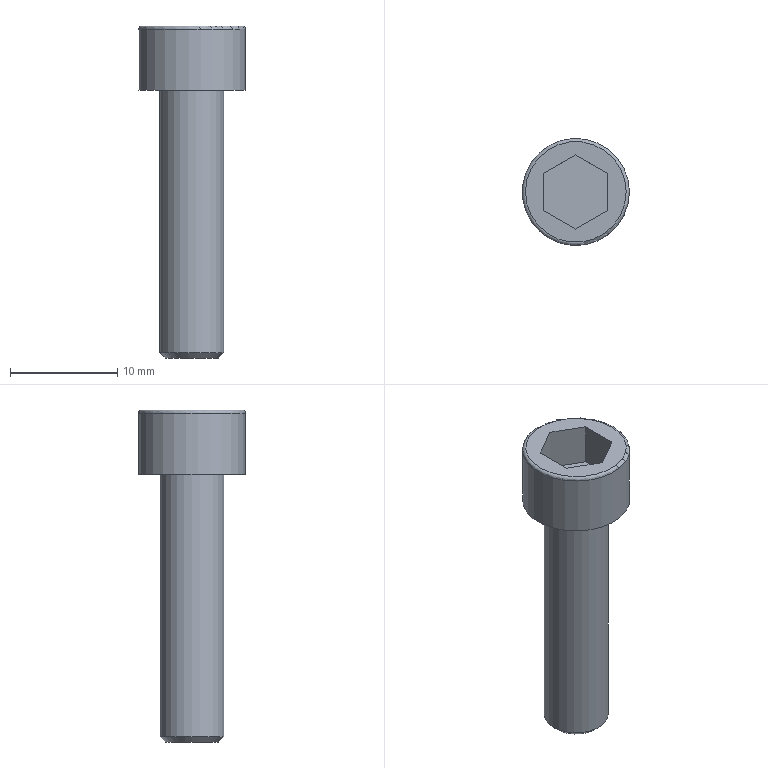Part | STEP file | 200 mesh_id622_x | 1 solid | 14 faces | box 10 x 10 x 31 mm | volume 1051 mm3 | plane 10 | cylinder 2 | torus 1 | cone 1 | commonest cylinder face diameters 6 x1 10 x1
STEP:
#1=CARTESIAN_POINT('',(-16735.684,-4117.769,77.5));
#2=VERTEX_POINT('',#1);
#3=CARTESIAN_POINT('',(-16732.684,-4117.769,77.5));
#4=DIRECTION('',(0.,0.,1.));
#5=DIRECTION('',(-1.,0.,0.));
#6=AXIS2_PLACEMENT_3D('',#3,#4,#5);
#7=CIRCLE('',#6,3.);
#8=EDGE_CURVE('',#2,#2,#7,.T.);
#9=ORIENTED_EDGE('',*,*,#8,.T.);
#10=EDGE_LOOP('',(#9));
#11=FACE_BOUND('',#10,.T.);
#12=CARTESIAN_POINT('',(-16735.684,-4117.769,102.));
#13=VERTEX_POINT('',#12);
#14=CARTESIAN_POINT('',(-16732.684,-4117.769,102.));
#15=DIRECTION('',(0.,0.,-1.));
#16=DIRECTION('',(-1.,0.,0.));
#17=AXIS2_PLACEMENT_3D('',#14,#15,#16);
#18=CIRCLE('',#17,3.);
#19=EDGE_CURVE('',#13,#13,#18,.T.);
#20=ORIENTED_EDGE('',*,*,#19,.T.);
#21=EDGE_LOOP('',(#20));
#22=FACE_BOUND('',#21,.T.);
#23=CARTESIAN_POINT('',(-16732.684,-4117.769,102.));
#24=DIRECTION('',(0.,0.,-1.));
#25=DIRECTION('',(1.,0.,0.));
#26=AXIS2_PLACEMENT_3D('',#23,#24,#25);
#27=CYLINDRICAL_SURFACE('',#26,3.);
#28=ADVANCED_FACE('',(#11,#22),#27,.T.);
#29=CARTESIAN_POINT('',(-16727.984,-4117.769,108.));
#30=VERTEX_POINT('',#29);
#31=CARTESIAN_POINT('',(-16732.684,-4117.769,108.));
#32=DIRECTION('',(0.,0.,-1.));
#33=DIRECTION('',(1.,0.,0.));
#34=AXIS2_PLACEMENT_3D('',#31,#32,#33);
#35=CIRCLE('',#34,4.7);
#36=EDGE_CURVE('',#30,#30,#35,.T.);
#37=ORIENTED_EDGE('',*,*,#36,.F.);
#38=EDGE_LOOP('',(#37));
#39=FACE_BOUND('',#38,.T.);
#40=CARTESIAN_POINT('',(-16735.684,-4119.501,108.));
#41=VERTEX_POINT('',#40);
#42=CARTESIAN_POINT('',(-16735.684,-4116.037,108.));
#43=VERTEX_POINT('',#42);
#44=CARTESIAN_POINT('',(-16735.684,-4119.501,108.));
#45=DIRECTION('',(0.,1.,0.));
#46=VECTOR('',#45,1.);
#47=LINE('',#44,#46);
#48=EDGE_CURVE('',#41,#43,#47,.T.);
#49=ORIENTED_EDGE('',*,*,#48,.T.);
#50=CARTESIAN_POINT('',(-16732.684,-4114.305,108.));
#51=VERTEX_POINT('',#50);
#52=CARTESIAN_POINT('',(-16735.684,-4116.037,108.));
#53=DIRECTION('',(0.866,0.5,0.));
#54=VECTOR('',#53,1.);
#55=LINE('',#52,#54);
#56=EDGE_CURVE('',#43,#51,#55,.T.);
#57=ORIENTED_EDGE('',*,*,#56,.T.);
#58=CARTESIAN_POINT('',(-16729.684,-4116.037,108.));
#59=VERTEX_POINT('',#58);
#60=CARTESIAN_POINT('',(-16732.684,-4114.305,108.));
#61=DIRECTION('',(0.866,-0.5,0.));
#62=VECTOR('',#61,1.);
#63=LINE('',#60,#62);
#64=EDGE_CURVE('',#51,#59,#63,.T.);
#65=ORIENTED_EDGE('',*,*,#64,.T.);
#66=CARTESIAN_POINT('',(-16729.684,-4119.501,108.));
#67=VERTEX_POINT('',#66);
#68=CARTESIAN_POINT('',(-16729.684,-4116.037,108.));
#69=DIRECTION('',(0.,-1.,0.));
#70=VECTOR('',#69,1.);
#71=LINE('',#68,#70);
#72=EDGE_CURVE('',#59,#67,#71,.T.);
#73=ORIENTED_EDGE('',*,*,#72,.T.);
#74=CARTESIAN_POINT('',(-16732.684,-4121.233,108.));
#75=VERTEX_POINT('',#74);
#76=CARTESIAN_POINT('',(-16729.684,-4119.501,108.));
#77=DIRECTION('',(-0.866,-0.5,0.));
#78=VECTOR('',#77,1.);
#79=LINE('',#76,#78);
#80=EDGE_CURVE('',#67,#75,#79,.T.);
#81=ORIENTED_EDGE('',*,*,#80,.T.);
#82=CARTESIAN_POINT('',(-16732.684,-4121.233,108.));
#83=DIRECTION('',(-0.866,0.5,0.));
#84=VECTOR('',#83,1.);
#85=LINE('',#82,#84);
#86=EDGE_CURVE('',#75,#41,#85,.T.);
#87=ORIENTED_EDGE('',*,*,#86,.T.);
#88=EDGE_LOOP('',(#49,#57,#65,#73,#81,#87));
#89=FACE_BOUND('',#88,.T.);
#90=CARTESIAN_POINT('',(-16732.684,-4117.769,108.));
#91=DIRECTION('',(0.,0.,1.));
#92=DIRECTION('',(1.,0.,0.));
#93=AXIS2_PLACEMENT_3D('',#90,#91,#92);
#94=PLANE('',#93);
#95=ADVANCED_FACE('',(#39,#89),#94,.T.);
#96=ORIENTED_EDGE('',*,*,#19,.F.);
#97=EDGE_LOOP('',(#96));
#98=FACE_BOUND('',#97,.T.);
#99=CARTESIAN_POINT('',(-16727.684,-4117.769,102.));
#100=VERTEX_POINT('',#99);
#101=CARTESIAN_POINT('',(-16732.684,-4117.769,102.));
#102=DIRECTION('',(0.,0.,-1.));
#103=DIRECTION('',(1.,0.,0.));
#104=AXIS2_PLACEMENT_3D('',#101,#102,#103);
#105=CIRCLE('',#104,5.);
#106=EDGE_CURVE('',#100,#100,#105,.T.);
#107=ORIENTED_EDGE('',*,*,#106,.T.);
#108=EDGE_LOOP('',(#107));
#109=FACE_BOUND('',#108,.T.);
#110=CARTESIAN_POINT('',(-16732.684,-4117.769,102.));
#111=DIRECTION('',(0.,0.,-1.));
#112=DIRECTION('',(-1.,0.,0.));
#113=AXIS2_PLACEMENT_3D('',#110,#111,#112);
#114=PLANE('',#113);
#115=ADVANCED_FACE('',(#98,#109),#114,.T.);
#116=CARTESIAN_POINT('',(-16727.684,-4117.769,107.7));
#117=VERTEX_POINT('',#116);
#118=CARTESIAN_POINT('',(-16732.684,-4117.769,107.7));
#119=DIRECTION('',(0.,0.,1.));
#120=DIRECTION('',(1.,0.,0.));
#121=AXIS2_PLACEMENT_3D('',#118,#119,#120);
#122=CIRCLE('',#121,5.);
#123=EDGE_CURVE('',#117,#117,#122,.T.);
#124=ORIENTED_EDGE('',*,*,#123,.F.);
#125=EDGE_LOOP('',(#124));
#126=FACE_BOUND('',#125,.T.);
#127=ORIENTED_EDGE('',*,*,#106,.F.);
#128=EDGE_LOOP('',(#127));
#129=FACE_BOUND('',#128,.T.);
#130=CARTESIAN_POINT('',(-16732.684,-4117.769,102.));
#131=DIRECTION('',(0.,0.,1.));
#132=DIRECTION('',(1.,0.,0.));
#133=AXIS2_PLACEMENT_3D('',#130,#131,#132);
#134=CYLINDRICAL_SURFACE('',#133,5.);
#135=ADVANCED_FACE('',(#126,#129),#134,.T.);
#136=CARTESIAN_POINT('',(-16735.684,-4116.037,104.));
#137=VERTEX_POINT('',#136);
#138=CARTESIAN_POINT('',(-16735.684,-4119.501,104.));
#139=VERTEX_POINT('',#138);
#140=CARTESIAN_POINT('',(-16735.684,-4119.501,104.));
#141=DIRECTION('',(0.,-1.,0.));
#142=VECTOR('',#141,1.);
#143=LINE('',#140,#142);
#144=EDGE_CURVE('',#137,#139,#143,.T.);
#145=ORIENTED_EDGE('',*,*,#144,.F.);
#146=CARTESIAN_POINT('',(-16735.684,-4116.037,108.));
#147=DIRECTION('',(0.,0.,1.));
#148=VECTOR('',#147,1.);
#149=LINE('',#146,#148);
#150=EDGE_CURVE('',#137,#43,#149,.T.);
#151=ORIENTED_EDGE('',*,*,#150,.T.);
#152=ORIENTED_EDGE('',*,*,#48,.F.);
#153=CARTESIAN_POINT('',(-16735.684,-4119.501,108.));
#154=DIRECTION('',(0.,0.,1.));
#155=VECTOR('',#154,1.);
#156=LINE('',#153,#155);
#157=EDGE_CURVE('',#139,#41,#156,.T.);
#158=ORIENTED_EDGE('',*,*,#157,.F.);
#159=EDGE_LOOP('',(#145,#151,#152,#158));
#160=FACE_OUTER_BOUND('',#159,.T.);
#161=CARTESIAN_POINT('',(-16735.684,-4119.501,108.));
#162=DIRECTION('',(1.,0.,0.));
#163=DIRECTION('',(0.,0.,-1.));
#164=AXIS2_PLACEMENT_3D('',#161,#162,#163);
#165=PLANE('',#164);
#166=ADVANCED_FACE('',(#160),#165,.T.);
#167=CARTESIAN_POINT('',(-16732.684,-4114.305,104.));
#168=VERTEX_POINT('',#167);
#169=CARTESIAN_POINT('',(-16735.684,-4116.037,104.));
#170=DIRECTION('',(-0.866,-0.5,0.));
#171=VECTOR('',#170,1.);
#172=LINE('',#169,#171);
#173=EDGE_CURVE('',#168,#137,#172,.T.);
#174=ORIENTED_EDGE('',*,*,#173,.F.);
#175=CARTESIAN_POINT('',(-16732.684,-4114.305,108.));
#176=DIRECTION('',(0.,0.,1.));
#177=VECTOR('',#176,1.);
#178=LINE('',#175,#177);
#179=EDGE_CURVE('',#168,#51,#178,.T.);
#180=ORIENTED_EDGE('',*,*,#179,.T.);
#181=ORIENTED_EDGE('',*,*,#56,.F.);
#182=ORIENTED_EDGE('',*,*,#150,.F.);
#183=EDGE_LOOP('',(#174,#180,#181,#182));
#184=FACE_OUTER_BOUND('',#183,.T.);
#185=CARTESIAN_POINT('',(-16735.684,-4116.037,108.));
#186=DIRECTION('',(0.5,-0.866,0.));
#187=DIRECTION('',(-0.866,-0.5,0.));
#188=AXIS2_PLACEMENT_3D('',#185,#186,#187);
#189=PLANE('',#188);
#190=ADVANCED_FACE('',(#184),#189,.T.);
#191=CARTESIAN_POINT('',(-16729.684,-4116.037,104.));
#192=VERTEX_POINT('',#191);
#193=CARTESIAN_POINT('',(-16732.684,-4114.305,104.));
#194=DIRECTION('',(-0.866,0.5,0.));
#195=VECTOR('',#194,1.);
#196=LINE('',#193,#195);
#197=EDGE_CURVE('',#192,#168,#196,.T.);
#198=ORIENTED_EDGE('',*,*,#197,.F.);
#199=CARTESIAN_POINT('',(-16729.684,-4116.037,108.));
#200=DIRECTION('',(0.,0.,1.));
#201=VECTOR('',#200,1.);
#202=LINE('',#199,#201);
#203=EDGE_CURVE('',#192,#59,#202,.T.);
#204=ORIENTED_EDGE('',*,*,#203,.T.);
#205=ORIENTED_EDGE('',*,*,#64,.F.);
#206=ORIENTED_EDGE('',*,*,#179,.F.);
#207=EDGE_LOOP('',(#198,#204,#205,#206));
#208=FACE_OUTER_BOUND('',#207,.T.);
#209=CARTESIAN_POINT('',(-16732.684,-4114.305,108.));
#210=DIRECTION('',(-0.5,-0.866,0.));
#211=DIRECTION('',(-0.866,0.5,0.));
#212=AXIS2_PLACEMENT_3D('',#209,#210,#211);
#213=PLANE('',#212);
#214=ADVANCED_FACE('',(#208),#213,.T.);
#215=CARTESIAN_POINT('',(-16729.684,-4119.501,104.));
#216=VERTEX_POINT('',#215);
#217=CARTESIAN_POINT('',(-16729.684,-4116.037,104.));
#218=DIRECTION('',(0.,1.,0.));
#219=VECTOR('',#218,1.);
#220=LINE('',#217,#219);
#221=EDGE_CURVE('',#216,#192,#220,.T.);
#222=ORIENTED_EDGE('',*,*,#221,.F.);
#223=CARTESIAN_POINT('',(-16729.684,-4119.501,108.));
#224=DIRECTION('',(0.,0.,1.));
#225=VECTOR('',#224,1.);
#226=LINE('',#223,#225);
#227=EDGE_CURVE('',#216,#67,#226,.T.);
#228=ORIENTED_EDGE('',*,*,#227,.T.);
#229=ORIENTED_EDGE('',*,*,#72,.F.);
#230=ORIENTED_EDGE('',*,*,#203,.F.);
#231=EDGE_LOOP('',(#222,#228,#229,#230));
#232=FACE_OUTER_BOUND('',#231,.T.);
#233=CARTESIAN_POINT('',(-16729.684,-4116.037,108.));
#234=DIRECTION('',(-1.,0.,0.));
#235=DIRECTION('',(0.,0.,1.));
#236=AXIS2_PLACEMENT_3D('',#233,#234,#235);
#237=PLANE('',#236);
#238=ADVANCED_FACE('',(#232),#237,.T.);
#239=CARTESIAN_POINT('',(-16732.684,-4121.233,104.));
#240=VERTEX_POINT('',#239);
#241=CARTESIAN_POINT('',(-16729.684,-4119.501,104.));
#242=DIRECTION('',(0.866,0.5,0.));
#243=VECTOR('',#242,1.);
#244=LINE('',#241,#243);
#245=EDGE_CURVE('',#240,#216,#244,.T.);
#246=ORIENTED_EDGE('',*,*,#245,.F.);
#247=CARTESIAN_POINT('',(-16732.684,-4121.233,108.));
#248=DIRECTION('',(0.,0.,1.));
#249=VECTOR('',#248,1.);
#250=LINE('',#247,#249);
#251=EDGE_CURVE('',#240,#75,#250,.T.);
#252=ORIENTED_EDGE('',*,*,#251,.T.);
#253=ORIENTED_EDGE('',*,*,#80,.F.);
#254=ORIENTED_EDGE('',*,*,#227,.F.);
#255=EDGE_LOOP('',(#246,#252,#253,#254));
#256=FACE_OUTER_BOUND('',#255,.T.);
#257=CARTESIAN_POINT('',(-16729.684,-4119.501,108.));
#258=DIRECTION('',(-0.5,0.866,0.));
#259=DIRECTION('',(0.866,0.5,0.));
#260=AXIS2_PLACEMENT_3D('',#257,#258,#259);
#261=PLANE('',#260);
#262=ADVANCED_FACE('',(#256),#261,.T.);
#263=CARTESIAN_POINT('',(-16732.684,-4121.233,104.));
#264=DIRECTION('',(0.866,-0.5,0.));
#265=VECTOR('',#264,1.);
#266=LINE('',#263,#265);
#267=EDGE_CURVE('',#139,#240,#266,.T.);
#268=ORIENTED_EDGE('',*,*,#267,.F.);
#269=ORIENTED_EDGE('',*,*,#157,.T.);
#270=ORIENTED_EDGE('',*,*,#86,.F.);
#271=ORIENTED_EDGE('',*,*,#251,.F.);
#272=EDGE_LOOP('',(#268,#269,#270,#271));
#273=FACE_OUTER_BOUND('',#272,.T.);
#274=CARTESIAN_POINT('',(-16732.684,-4121.233,108.));
#275=DIRECTION('',(0.5,0.866,0.));
#276=DIRECTION('',(0.866,-0.5,0.));
#277=AXIS2_PLACEMENT_3D('',#274,#275,#276);
#278=PLANE('',#277);
#279=ADVANCED_FACE('',(#273),#278,.T.);
#280=ORIENTED_EDGE('',*,*,#144,.T.);
#281=ORIENTED_EDGE('',*,*,#267,.T.);
#282=ORIENTED_EDGE('',*,*,#245,.T.);
#283=ORIENTED_EDGE('',*,*,#221,.T.);
#284=ORIENTED_EDGE('',*,*,#197,.T.);
#285=ORIENTED_EDGE('',*,*,#173,.T.);
#286=EDGE_LOOP('',(#280,#281,#282,#283,#284,#285));
#287=FACE_OUTER_BOUND('',#286,.T.);
#288=CARTESIAN_POINT('',(-22.998,-8288.038,104.));
#289=DIRECTION('',(0.,0.,1.));
#290=DIRECTION('',(1.,0.,0.));
#291=AXIS2_PLACEMENT_3D('',#288,#289,#290);
#292=PLANE('',#291);
#293=ADVANCED_FACE('',(#287),#292,.T.);
#294=ORIENTED_EDGE('',*,*,#36,.T.);
#295=EDGE_LOOP('',(#294));
#296=FACE_BOUND('',#295,.T.);
#297=ORIENTED_EDGE('',*,*,#123,.T.);
#298=EDGE_LOOP('',(#297));
#299=FACE_BOUND('',#298,.T.);
#300=CARTESIAN_POINT('',(-16732.684,-4117.769,107.7));
#301=DIRECTION('',(0.,0.,1.));
#302=DIRECTION('',(1.,0.,0.));
#303=AXIS2_PLACEMENT_3D('',#300,#301,#302);
#304=TOROIDAL_SURFACE('',#303,4.7,0.3);
#305=ADVANCED_FACE('',(#296,#299),#304,.T.);
#306=CARTESIAN_POINT('',(-16735.184,-4117.769,77.));
#307=VERTEX_POINT('',#306);
#308=CARTESIAN_POINT('',(-16732.684,-4117.769,77.));
#309=DIRECTION('',(0.,0.,-1.));
#310=DIRECTION('',(-1.,0.,0.));
#311=AXIS2_PLACEMENT_3D('',#308,#309,#310);
#312=CIRCLE('',#311,2.5);
#313=EDGE_CURVE('',#307,#307,#312,.T.);
#314=ORIENTED_EDGE('',*,*,#313,.T.);
#315=EDGE_LOOP('',(#314));
#316=FACE_OUTER_BOUND('',#315,.T.);
#317=CARTESIAN_POINT('',(-16732.684,-4117.769,77.));
#318=DIRECTION('',(0.,0.,-1.));
#319=DIRECTION('',(-1.,0.,0.));
#320=AXIS2_PLACEMENT_3D('',#317,#318,#319);
#321=PLANE('',#320);
#322=ADVANCED_FACE('',(#316),#321,.T.);
#323=ORIENTED_EDGE('',*,*,#313,.F.);
#324=EDGE_LOOP('',(#323));
#325=FACE_BOUND('',#324,.T.);
#326=ORIENTED_EDGE('',*,*,#8,.F.);
#327=EDGE_LOOP('',(#326));
#328=FACE_BOUND('',#327,.T.);
#329=CARTESIAN_POINT('',(-16732.684,-4117.769,77.5));
#330=DIRECTION('',(0.,0.,1.));
#331=DIRECTION('',(1.,0.,0.));
#332=AXIS2_PLACEMENT_3D('',#329,#330,#331);
#333=CONICAL_SURFACE('',#332,3.,45.);
#334=ADVANCED_FACE('',(#325,#328),#333,.T.);
#335=CLOSED_SHELL('',(#28,#95,#115,#135,#166,#190,#214,#238,#262,#279,#293,#305,#322,#334));
#336=MANIFOLD_SOLID_BREP('',#335);
#337=(LENGTH_UNIT()NAMED_UNIT(*)SI_UNIT(.MILLI.,.METRE.));
#338=UNCERTAINTY_MEASURE_WITH_UNIT(LENGTH_MEASURE(0.00002),#337,'','');
#339=(NAMED_UNIT(*)PLANE_ANGLE_UNIT()SI_UNIT($,.RADIAN.));
#340=PLANE_ANGLE_MEASURE_WITH_UNIT(PLANE_ANGLE_MEASURE(0.01745),#339);
#341=DIMENSIONAL_EXPONENTS(0.,0.,0.,0.,0.,0.,0.);
#342=(CONVERSION_BASED_UNIT('DEGREE',#340)NAMED_UNIT(#341)PLANE_ANGLE_UNIT());
#343=(NAMED_UNIT(*)SI_UNIT($,.STERADIAN.)SOLID_ANGLE_UNIT());
#344=(GEOMETRIC_REPRESENTATION_CONTEXT(3)GLOBAL_UNCERTAINTY_ASSIGNED_CONTEXT((#338))GLOBAL_UNIT_ASSIGNED_CONTEXT((#337,#342,#343))REPRESENTATION_CONTEXT('',''));
#345=ADVANCED_BREP_SHAPE_REPRESENTATION('',(#336),#344);